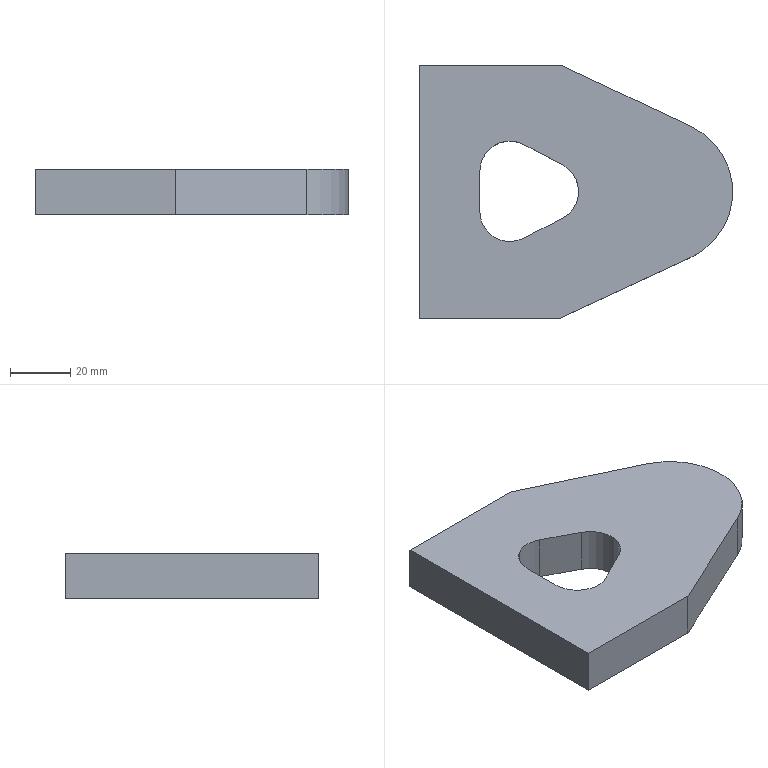Part | STEP file | ASND-0110-BAIF-08 | 1 solid | 16 faces | box 104 x 84 x 15 mm | volume 94605 mm3 | plane 10 | cylinder 6 | commonest cylinder face diameters 20 x5 48 x1
STEP:
#1=CARTESIAN_POINT('',(0.,0.,0.));
#2=DIRECTION('',(0.,0.,1.));
#3=DIRECTION('',(1.,0.,0.));
#4=AXIS2_PLACEMENT_3D('',#1,#2,#3);
#5=CARTESIAN_POINT('',(55.,6.858,20.));
#6=VERTEX_POINT('',#5);
#7=CARTESIAN_POINT('',(55.,6.858,5.));
#8=VERTEX_POINT('',#7);
#9=CARTESIAN_POINT('',(55.,6.858,0.));
#10=DIRECTION('',(0.,0.,-1.));
#11=VECTOR('',#10,1.);
#12=LINE('',#9,#11);
#13=CARTESIAN_POINT('',(65.,6.858,0.));
#14=DIRECTION('',(0.,0.,1.));
#15=DIRECTION('',(-0.5173,0.8558,0.));
#16=AXIS2_PLACEMENT_3D('',#13,#14,#15);
#17=CYLINDRICAL_SURFACE('',#16,10.);
#18=CARTESIAN_POINT('',(1.027,0.));
#19=DIRECTION('',(0.,-1.));
#20=VECTOR('',#19,1.);
#21=LINE('',#18,#20);
#22=(GEOMETRIC_REPRESENTATION_CONTEXT(2)PARAMETRIC_REPRESENTATION_CONTEXT()REPRESENTATION_CONTEXT('',''));
#23=DEFINITIONAL_REPRESENTATION('',(#21),#22);
#24=PCURVE('',#17,#23);
#25=CARTESIAN_POINT('',(55.,57.525,0.));
#26=DIRECTION('',(-1.,0.,0.));
#27=DIRECTION('',(0.,0.7071,0.7071));
#28=AXIS2_PLACEMENT_3D('',#25,#26,#27);
#29=PLANE('',#28);
#30=CARTESIAN_POINT('',(-35.827,-35.827));
#31=DIRECTION('',(-0.7071,0.7071));
#32=VECTOR('',#31,1.);
#33=LINE('',#30,#32);
#34=(GEOMETRIC_REPRESENTATION_CONTEXT(2)PARAMETRIC_REPRESENTATION_CONTEXT()REPRESENTATION_CONTEXT('',''));
#35=DEFINITIONAL_REPRESENTATION('',(#33),#34);
#36=PCURVE('',#29,#35);
#37=SURFACE_CURVE('',#12,(#24,#36),.PCURVE_S1.);
#38=EDGE_CURVE('',#6,#8,#37,.T.);
#39=ORIENTED_EDGE('',*,*,#38,.F.);
#40=CARTESIAN_POINT('',(59.827,15.416,20.));
#41=VERTEX_POINT('',#40);
#42=CARTESIAN_POINT('',(65.,6.858,20.));
#43=DIRECTION('',(0.,0.,1.));
#44=DIRECTION('',(-0.5173,0.8558,0.));
#45=AXIS2_PLACEMENT_3D('',#42,#43,#44);
#46=CIRCLE('',#45,10.);
#47=CARTESIAN_POINT('',(0.,20.));
#48=DIRECTION('',(1.,0.));
#49=VECTOR('',#48,1.);
#50=LINE('',#47,#49);
#51=(GEOMETRIC_REPRESENTATION_CONTEXT(2)PARAMETRIC_REPRESENTATION_CONTEXT()REPRESENTATION_CONTEXT('',''));
#52=DEFINITIONAL_REPRESENTATION('',(#50),#51);
#53=PCURVE('',#17,#52);
#54=CARTESIAN_POINT('',(115.,0.,20.));
#55=DIRECTION('',(0.,0.,1.));
#56=DIRECTION('',(0.7071,0.7071,0.));
#57=AXIS2_PLACEMENT_3D('',#54,#55,#56);
#58=PLANE('',#57);
#59=CARTESIAN_POINT('',(-30.506,40.205));
#60=DIRECTION('',(0.2394,0.9709));
#61=AXIS2_PLACEMENT_2D('',#59,#60);
#62=CIRCLE('',#61,10.);
#63=(GEOMETRIC_REPRESENTATION_CONTEXT(2)PARAMETRIC_REPRESENTATION_CONTEXT()REPRESENTATION_CONTEXT('',''));
#64=DEFINITIONAL_REPRESENTATION('',(#62),#63);
#65=PCURVE('',#58,#64);
#66=SURFACE_CURVE('',#46,(#53,#65),.PCURVE_S1.);
#67=EDGE_CURVE('',#41,#6,#66,.T.);
#68=ORIENTED_EDGE('',*,*,#67,.F.);
#69=CARTESIAN_POINT('',(59.827,15.416,5.));
#70=VERTEX_POINT('',#69);
#71=CARTESIAN_POINT('',(59.827,15.416,0.));
#72=DIRECTION('',(0.,0.,1.));
#73=VECTOR('',#72,1.);
#74=LINE('',#71,#73);
#75=CARTESIAN_POINT('',(0.,0.));
#76=DIRECTION('',(0.,1.));
#77=VECTOR('',#76,1.);
#78=LINE('',#75,#77);
#79=(GEOMETRIC_REPRESENTATION_CONTEXT(2)PARAMETRIC_REPRESENTATION_CONTEXT()REPRESENTATION_CONTEXT('',''));
#80=DEFINITIONAL_REPRESENTATION('',(#78),#79);
#81=PCURVE('',#17,#80);
#82=CARTESIAN_POINT('',(65.,6.858,0.));
#83=DIRECTION('',(0.,0.,1.));
#84=DIRECTION('',(-0.5173,0.8558,0.));
#85=AXIS2_PLACEMENT_3D('',#82,#83,#84);
#86=CYLINDRICAL_SURFACE('',#85,10.);
#87=CARTESIAN_POINT('',(6.283,0.));
#88=DIRECTION('',(0.,1.));
#89=VECTOR('',#88,1.);
#90=LINE('',#87,#89);
#91=(GEOMETRIC_REPRESENTATION_CONTEXT(2)PARAMETRIC_REPRESENTATION_CONTEXT()REPRESENTATION_CONTEXT('',''));
#92=DEFINITIONAL_REPRESENTATION('',(#90),#91);
#93=PCURVE('',#86,#92);
#94=SURFACE_CURVE('',#74,(#81,#93),.PCURVE_S1.);
#95=EDGE_CURVE('',#70,#41,#94,.T.);
#96=ORIENTED_EDGE('',*,*,#95,.F.);
#97=CARTESIAN_POINT('',(65.,6.858,5.));
#98=DIRECTION('',(0.,0.,-1.));
#99=DIRECTION('',(-0.5173,0.8558,0.));
#100=AXIS2_PLACEMENT_3D('',#97,#98,#99);
#101=CIRCLE('',#100,10.);
#102=CARTESIAN_POINT('',(6.283,5.));
#103=DIRECTION('',(-1.,0.));
#104=VECTOR('',#103,1.);
#105=LINE('',#102,#104);
#106=(GEOMETRIC_REPRESENTATION_CONTEXT(2)PARAMETRIC_REPRESENTATION_CONTEXT()REPRESENTATION_CONTEXT('',''));
#107=DEFINITIONAL_REPRESENTATION('',(#105),#106);
#108=PCURVE('',#17,#107);
#109=CARTESIAN_POINT('',(115.,0.,5.));
#110=DIRECTION('',(0.,0.,1.));
#111=DIRECTION('',(0.7071,0.7071,0.));
#112=AXIS2_PLACEMENT_3D('',#109,#110,#111);
#113=PLANE('',#112);
#114=CARTESIAN_POINT('',(-28.113,49.914));
#115=CARTESIAN_POINT('',(-11.296,45.768));
#116=CARTESIAN_POINT('',(-23.294,33.277));
#117=CARTESIAN_POINT('',(-35.293,20.786));
#118=CARTESIAN_POINT('',(-40.111,37.423));
#119=CARTESIAN_POINT('',(-44.93,54.06));
#120=CARTESIAN_POINT('',(-28.113,49.914));
#121=(BOUNDED_CURVE()B_SPLINE_CURVE(2,(#114,#115,#116,#117,#118,#119,#120),.UNSPECIFIED.,.T.,.F.)B_SPLINE_CURVE_WITH_KNOTS((1,2,2,2,2,1),(-2.094,0.,2.094,4.189,6.283,8.378),.UNSPECIFIED.)CURVE()GEOMETRIC_REPRESENTATION_ITEM()RATIONAL_B_SPLINE_CURVE((1.,0.5,1.,0.5,1.,0.5,1.))REPRESENTATION_ITEM(''));
#122=(GEOMETRIC_REPRESENTATION_CONTEXT(2)PARAMETRIC_REPRESENTATION_CONTEXT()REPRESENTATION_CONTEXT('',''));
#123=DEFINITIONAL_REPRESENTATION('',(#121),#122);
#124=PCURVE('',#113,#123);
#125=SURFACE_CURVE('',#101,(#108,#124),.PCURVE_S1.);
#126=EDGE_CURVE('',#8,#70,#125,.T.);
#127=ORIENTED_EDGE('',*,*,#126,.F.);
#128=EDGE_LOOP('',(#39,#68,#96,#127));
#129=FACE_BOUND('',#128,.F.);
#130=ADVANCED_FACE('',(#129),#17,.F.);
#131=CARTESIAN_POINT('',(55.,-6.459,5.));
#132=VERTEX_POINT('',#131);
#133=CARTESIAN_POINT('',(55.,-6.459,20.));
#134=VERTEX_POINT('',#133);
#135=CARTESIAN_POINT('',(55.,-6.459,0.));
#136=DIRECTION('',(0.,0.,1.));
#137=VECTOR('',#136,1.);
#138=LINE('',#135,#137);
#139=CARTESIAN_POINT('',(65.,-6.459,0.));
#140=DIRECTION('',(0.,0.,-1.));
#141=DIRECTION('',(-0.5205,-0.8539,0.));
#142=AXIS2_PLACEMENT_3D('',#139,#140,#141);
#143=CYLINDRICAL_SURFACE('',#142,10.);
#144=CARTESIAN_POINT('',(1.023,0.));
#145=DIRECTION('',(0.,-1.));
#146=VECTOR('',#145,1.);
#147=LINE('',#144,#146);
#148=(GEOMETRIC_REPRESENTATION_CONTEXT(2)PARAMETRIC_REPRESENTATION_CONTEXT()REPRESENTATION_CONTEXT('',''));
#149=DEFINITIONAL_REPRESENTATION('',(#147),#148);
#150=PCURVE('',#143,#149);
#151=CARTESIAN_POINT('',(-45.244,-45.244));
#152=DIRECTION('',(0.7071,-0.7071));
#153=VECTOR('',#152,1.);
#154=LINE('',#151,#153);
#155=(GEOMETRIC_REPRESENTATION_CONTEXT(2)PARAMETRIC_REPRESENTATION_CONTEXT()REPRESENTATION_CONTEXT('',''));
#156=DEFINITIONAL_REPRESENTATION('',(#154),#155);
#157=PCURVE('',#29,#156);
#158=SURFACE_CURVE('',#138,(#150,#157),.PCURVE_S1.);
#159=EDGE_CURVE('',#132,#134,#158,.T.);
#160=ORIENTED_EDGE('',*,*,#159,.F.);
#161=CARTESIAN_POINT('',(59.795,-14.998,5.));
#162=VERTEX_POINT('',#161);
#163=CARTESIAN_POINT('',(65.,-6.459,5.));
#164=DIRECTION('',(0.,0.,-1.));
#165=DIRECTION('',(-0.5205,-0.8539,0.));
#166=AXIS2_PLACEMENT_3D('',#163,#164,#165);
#167=CIRCLE('',#166,10.);
#168=CARTESIAN_POINT('',(0.,-5.));
#169=DIRECTION('',(1.,0.));
#170=VECTOR('',#169,1.);
#171=LINE('',#168,#170);
#172=(GEOMETRIC_REPRESENTATION_CONTEXT(2)PARAMETRIC_REPRESENTATION_CONTEXT()REPRESENTATION_CONTEXT('',''));
#173=DEFINITIONAL_REPRESENTATION('',(#171),#172);
#174=PCURVE('',#143,#173);
#175=CARTESIAN_POINT('',(-49.641,28.431));
#176=CARTESIAN_POINT('',(-53.724,45.263));
#177=CARTESIAN_POINT('',(-37.105,40.383));
#178=CARTESIAN_POINT('',(-20.486,35.502));
#179=CARTESIAN_POINT('',(-33.022,23.55));
#180=CARTESIAN_POINT('',(-45.558,11.598));
#181=CARTESIAN_POINT('',(-49.641,28.431));
#182=(BOUNDED_CURVE()B_SPLINE_CURVE(2,(#175,#176,#177,#178,#179,#180,#181),.UNSPECIFIED.,.T.,.F.)B_SPLINE_CURVE_WITH_KNOTS((1,2,2,2,2,1),(-2.094,0.,2.094,4.189,6.283,8.378),.UNSPECIFIED.)CURVE()GEOMETRIC_REPRESENTATION_ITEM()RATIONAL_B_SPLINE_CURVE((1.,0.5,1.,0.5,1.,0.5,1.))REPRESENTATION_ITEM(''));
#183=(GEOMETRIC_REPRESENTATION_CONTEXT(2)PARAMETRIC_REPRESENTATION_CONTEXT()REPRESENTATION_CONTEXT('',''));
#184=DEFINITIONAL_REPRESENTATION('',(#182),#183);
#185=PCURVE('',#113,#184);
#186=SURFACE_CURVE('',#167,(#174,#185),.PCURVE_S1.);
#187=EDGE_CURVE('',#162,#132,#186,.T.);
#188=ORIENTED_EDGE('',*,*,#187,.F.);
#189=CARTESIAN_POINT('',(59.795,-14.998,20.));
#190=VERTEX_POINT('',#189);
#191=CARTESIAN_POINT('',(59.795,-14.998,0.));
#192=DIRECTION('',(0.,0.,-1.));
#193=VECTOR('',#192,1.);
#194=LINE('',#191,#193);
#195=CARTESIAN_POINT('',(0.,0.));
#196=DIRECTION('',(0.,1.));
#197=VECTOR('',#196,1.);
#198=LINE('',#195,#197);
#199=(GEOMETRIC_REPRESENTATION_CONTEXT(2)PARAMETRIC_REPRESENTATION_CONTEXT()REPRESENTATION_CONTEXT('',''));
#200=DEFINITIONAL_REPRESENTATION('',(#198),#199);
#201=PCURVE('',#143,#200);
#202=CARTESIAN_POINT('',(65.,-6.459,0.));
#203=DIRECTION('',(0.,0.,-1.));
#204=DIRECTION('',(-0.5205,-0.8539,0.));
#205=AXIS2_PLACEMENT_3D('',#202,#203,#204);
#206=CYLINDRICAL_SURFACE('',#205,10.);
#207=CARTESIAN_POINT('',(6.283,0.));
#208=DIRECTION('',(0.,1.));
#209=VECTOR('',#208,1.);
#210=LINE('',#207,#209);
#211=(GEOMETRIC_REPRESENTATION_CONTEXT(2)PARAMETRIC_REPRESENTATION_CONTEXT()REPRESENTATION_CONTEXT('',''));
#212=DEFINITIONAL_REPRESENTATION('',(#210),#211);
#213=PCURVE('',#206,#212);
#214=SURFACE_CURVE('',#194,(#201,#213),.PCURVE_S1.);
#215=EDGE_CURVE('',#190,#162,#214,.T.);
#216=ORIENTED_EDGE('',*,*,#215,.F.);
#217=CARTESIAN_POINT('',(65.,-6.459,20.));
#218=DIRECTION('',(0.,0.,1.));
#219=DIRECTION('',(-0.5205,-0.8539,0.));
#220=AXIS2_PLACEMENT_3D('',#217,#218,#219);
#221=CIRCLE('',#220,10.);
#222=CARTESIAN_POINT('',(6.283,-20.));
#223=DIRECTION('',(-1.,0.));
#224=VECTOR('',#223,1.);
#225=LINE('',#222,#224);
#226=(GEOMETRIC_REPRESENTATION_CONTEXT(2)PARAMETRIC_REPRESENTATION_CONTEXT()REPRESENTATION_CONTEXT('',''));
#227=DEFINITIONAL_REPRESENTATION('',(#225),#226);
#228=PCURVE('',#143,#227);
#229=CARTESIAN_POINT('',(-39.923,30.788));
#230=DIRECTION('',(-0.9718,-0.2357));
#231=AXIS2_PLACEMENT_2D('',#229,#230);
#232=CIRCLE('',#231,10.);
#233=(GEOMETRIC_REPRESENTATION_CONTEXT(2)PARAMETRIC_REPRESENTATION_CONTEXT()REPRESENTATION_CONTEXT('',''));
#234=DEFINITIONAL_REPRESENTATION('',(#232),#233);
#235=PCURVE('',#58,#234);
#236=SURFACE_CURVE('',#221,(#228,#235),.PCURVE_S1.);
#237=EDGE_CURVE('',#134,#190,#236,.T.);
#238=ORIENTED_EDGE('',*,*,#237,.F.);
#239=EDGE_LOOP('',(#160,#188,#216,#238));
#240=FACE_BOUND('',#239,.F.);
#241=ADVANCED_FACE('',(#240),#143,.F.);
#242=CARTESIAN_POINT('',(82.175,42.,20.));
#243=VERTEX_POINT('',#242);
#244=CARTESIAN_POINT('',(125.231,21.71,20.));
#245=VERTEX_POINT('',#244);
#246=CARTESIAN_POINT('',(71.564,47.,20.));
#247=DIRECTION('',(0.9046,-0.4263,0.));
#248=VECTOR('',#247,1.);
#249=LINE('',#246,#248);
#250=CARTESIAN_POINT('',(71.564,47.,5.));
#251=DIRECTION('',(0.4263,0.9046,0.));
#252=DIRECTION('',(0.6708,-0.3161,0.6708));
#253=AXIS2_PLACEMENT_3D('',#250,#251,#252);
#254=PLANE('',#253);
#255=CARTESIAN_POINT('',(10.063,-11.124));
#256=DIRECTION('',(0.7416,0.6708));
#257=VECTOR('',#256,1.);
#258=LINE('',#255,#257);
#259=(GEOMETRIC_REPRESENTATION_CONTEXT(2)PARAMETRIC_REPRESENTATION_CONTEXT()REPRESENTATION_CONTEXT('',''));
#260=DEFINITIONAL_REPRESENTATION('',(#258),#259);
#261=PCURVE('',#254,#260);
#262=CARTESIAN_POINT('',(2.52,63.948));
#263=DIRECTION('',(0.3382,-0.9411));
#264=VECTOR('',#263,1.);
#265=LINE('',#262,#264);
#266=(GEOMETRIC_REPRESENTATION_CONTEXT(2)PARAMETRIC_REPRESENTATION_CONTEXT()REPRESENTATION_CONTEXT('',''));
#267=DEFINITIONAL_REPRESENTATION('',(#265),#266);
#268=PCURVE('',#58,#267);
#269=SURFACE_CURVE('',#249,(#261,#268),.PCURVE_S1.);
#270=EDGE_CURVE('',#243,#245,#269,.T.);
#271=ORIENTED_EDGE('',*,*,#270,.T.);
#272=CARTESIAN_POINT('',(125.231,21.71,5.));
#273=VERTEX_POINT('',#272);
#274=CARTESIAN_POINT('',(125.231,21.71,5.));
#275=DIRECTION('',(0.,0.,1.));
#276=VECTOR('',#275,1.);
#277=LINE('',#274,#276);
#278=CARTESIAN_POINT('',(43.997,39.799));
#279=DIRECTION('',(0.6708,-0.7416));
#280=VECTOR('',#279,1.);
#281=LINE('',#278,#280);
#282=(GEOMETRIC_REPRESENTATION_CONTEXT(2)PARAMETRIC_REPRESENTATION_CONTEXT()REPRESENTATION_CONTEXT('',''));
#283=DEFINITIONAL_REPRESENTATION('',(#281),#282);
#284=PCURVE('',#254,#283);
#285=CARTESIAN_POINT('',(115.,0.,5.));
#286=DIRECTION('',(0.,0.,1.));
#287=DIRECTION('',(-1.,0.,0.));
#288=AXIS2_PLACEMENT_3D('',#285,#286,#287);
#289=CYLINDRICAL_SURFACE('',#288,24.);
#290=CARTESIAN_POINT('',(4.272,0.));
#291=DIRECTION('',(0.,1.));
#292=VECTOR('',#291,1.);
#293=LINE('',#290,#292);
#294=(GEOMETRIC_REPRESENTATION_CONTEXT(2)PARAMETRIC_REPRESENTATION_CONTEXT()REPRESENTATION_CONTEXT('',''));
#295=DEFINITIONAL_REPRESENTATION('',(#293),#294);
#296=PCURVE('',#289,#295);
#297=SURFACE_CURVE('',#277,(#284,#296),.PCURVE_S1.);
#298=EDGE_CURVE('',#273,#245,#297,.T.);
#299=ORIENTED_EDGE('',*,*,#298,.F.);
#300=CARTESIAN_POINT('',(82.175,42.,5.));
#301=VERTEX_POINT('',#300);
#302=CARTESIAN_POINT('',(71.564,47.,5.));
#303=DIRECTION('',(0.9046,-0.4263,0.));
#304=VECTOR('',#303,1.);
#305=LINE('',#302,#304);
#306=CARTESIAN_POINT('',(0.,0.));
#307=DIRECTION('',(0.7416,0.6708));
#308=VECTOR('',#307,1.);
#309=LINE('',#306,#308);
#310=(GEOMETRIC_REPRESENTATION_CONTEXT(2)PARAMETRIC_REPRESENTATION_CONTEXT()REPRESENTATION_CONTEXT('',''));
#311=DEFINITIONAL_REPRESENTATION('',(#309),#310);
#312=PCURVE('',#254,#311);
#313=CARTESIAN_POINT('',(2.52,63.948));
#314=DIRECTION('',(0.3382,-0.9411));
#315=VECTOR('',#314,1.);
#316=LINE('',#313,#315);
#317=(GEOMETRIC_REPRESENTATION_CONTEXT(2)PARAMETRIC_REPRESENTATION_CONTEXT()REPRESENTATION_CONTEXT('',''));
#318=DEFINITIONAL_REPRESENTATION('',(#316),#317);
#319=PCURVE('',#113,#318);
#320=SURFACE_CURVE('',#305,(#312,#319),.PCURVE_S1.);
#321=EDGE_CURVE('',#301,#273,#320,.T.);
#322=ORIENTED_EDGE('',*,*,#321,.F.);
#323=CARTESIAN_POINT('',(82.175,42.,12.5));
#324=DIRECTION('',(0.,0.,-1.));
#325=VECTOR('',#324,1.);
#326=LINE('',#323,#325);
#327=CARTESIAN_POINT('',(13.73,2.307));
#328=DIRECTION('',(-0.6708,0.7416));
#329=VECTOR('',#328,1.);
#330=LINE('',#327,#329);
#331=(GEOMETRIC_REPRESENTATION_CONTEXT(2)PARAMETRIC_REPRESENTATION_CONTEXT()REPRESENTATION_CONTEXT('',''));
#332=DEFINITIONAL_REPRESENTATION('',(#330),#331);
#333=PCURVE('',#254,#332);
#334=CARTESIAN_POINT('',(10.,42.,20.));
#335=DIRECTION('',(0.,-1.,0.));
#336=DIRECTION('',(0.7071,0.,0.7071));
#337=AXIS2_PLACEMENT_3D('',#334,#335,#336);
#338=PLANE('',#337);
#339=CARTESIAN_POINT('',(45.732,-56.339));
#340=DIRECTION('',(-0.7071,-0.7071));
#341=VECTOR('',#340,1.);
#342=LINE('',#339,#341);
#343=(GEOMETRIC_REPRESENTATION_CONTEXT(2)PARAMETRIC_REPRESENTATION_CONTEXT()REPRESENTATION_CONTEXT('',''));
#344=DEFINITIONAL_REPRESENTATION('',(#342),#343);
#345=PCURVE('',#338,#344);
#346=SURFACE_CURVE('',#326,(#333,#345),.PCURVE_S1.);
#347=EDGE_CURVE('',#243,#301,#346,.T.);
#348=ORIENTED_EDGE('',*,*,#347,.F.);
#349=EDGE_LOOP('',(#271,#299,#322,#348));
#350=FACE_BOUND('',#349,.T.);
#351=ADVANCED_FACE('',(#350),#254,.T.);
#352=CARTESIAN_POINT('',(125.104,-21.77,20.));
#353=VERTEX_POINT('',#352);
#354=CARTESIAN_POINT('',(115.,0.,20.));
#355=DIRECTION('',(0.,0.,-1.));
#356=DIRECTION('',(-1.,0.,0.));
#357=AXIS2_PLACEMENT_3D('',#354,#355,#356);
#358=CIRCLE('',#357,24.);
#359=CARTESIAN_POINT('',(6.283,15.));
#360=DIRECTION('',(-1.,0.));
#361=VECTOR('',#360,1.);
#362=LINE('',#359,#361);
#363=(GEOMETRIC_REPRESENTATION_CONTEXT(2)PARAMETRIC_REPRESENTATION_CONTEXT()REPRESENTATION_CONTEXT('',''));
#364=DEFINITIONAL_REPRESENTATION('',(#362),#363);
#365=PCURVE('',#289,#364);
#366=CARTESIAN_POINT('',(-16.971,16.971));
#367=CARTESIAN_POINT('',(12.423,46.364));
#368=CARTESIAN_POINT('',(23.182,6.212));
#369=CARTESIAN_POINT('',(33.941,-33.941));
#370=CARTESIAN_POINT('',(-6.212,-23.182));
#371=CARTESIAN_POINT('',(-46.364,-12.423));
#372=CARTESIAN_POINT('',(-16.971,16.971));
#373=(BOUNDED_CURVE()B_SPLINE_CURVE(2,(#366,#367,#368,#369,#370,#371,#372),.UNSPECIFIED.,.T.,.F.)B_SPLINE_CURVE_WITH_KNOTS((1,2,2,2,2,1),(-2.094,0.,2.094,4.189,6.283,8.378),.UNSPECIFIED.)CURVE()GEOMETRIC_REPRESENTATION_ITEM()RATIONAL_B_SPLINE_CURVE((1.,0.5,1.,0.5,1.,0.5,1.))REPRESENTATION_ITEM(''));
#374=(GEOMETRIC_REPRESENTATION_CONTEXT(2)PARAMETRIC_REPRESENTATION_CONTEXT()REPRESENTATION_CONTEXT('',''));
#375=DEFINITIONAL_REPRESENTATION('',(#373),#374);
#376=PCURVE('',#58,#375);
#377=SURFACE_CURVE('',#358,(#365,#376),.PCURVE_S1.);
#378=EDGE_CURVE('',#245,#353,#377,.T.);
#379=ORIENTED_EDGE('',*,*,#378,.T.);
#380=CARTESIAN_POINT('',(125.104,-21.77,5.));
#381=VERTEX_POINT('',#380);
#382=CARTESIAN_POINT('',(125.104,-21.77,5.));
#383=DIRECTION('',(0.,0.,1.));
#384=VECTOR('',#383,1.);
#385=LINE('',#382,#384);
#386=CARTESIAN_POINT('',(2.005,0.));
#387=DIRECTION('',(0.,1.));
#388=VECTOR('',#387,1.);
#389=LINE('',#386,#388);
#390=(GEOMETRIC_REPRESENTATION_CONTEXT(2)PARAMETRIC_REPRESENTATION_CONTEXT()REPRESENTATION_CONTEXT('',''));
#391=DEFINITIONAL_REPRESENTATION('',(#389),#390);
#392=PCURVE('',#289,#391);
#393=CARTESIAN_POINT('',(125.104,-21.77,5.));
#394=DIRECTION('',(0.421,-0.9071,0.));
#395=DIRECTION('',(0.6719,0.3118,0.6719));
#396=AXIS2_PLACEMENT_3D('',#393,#394,#395);
#397=PLANE('',#396);
#398=CARTESIAN_POINT('',(0.,0.));
#399=DIRECTION('',(0.6719,0.7407));
#400=VECTOR('',#399,1.);
#401=LINE('',#398,#400);
#402=(GEOMETRIC_REPRESENTATION_CONTEXT(2)PARAMETRIC_REPRESENTATION_CONTEXT()REPRESENTATION_CONTEXT('',''));
#403=DEFINITIONAL_REPRESENTATION('',(#401),#402);
#404=PCURVE('',#397,#403);
#405=SURFACE_CURVE('',#385,(#392,#404),.PCURVE_S1.);
#406=EDGE_CURVE('',#381,#353,#405,.T.);
#407=ORIENTED_EDGE('',*,*,#406,.F.);
#408=CARTESIAN_POINT('',(115.,0.,5.));
#409=DIRECTION('',(0.,0.,-1.));
#410=DIRECTION('',(-1.,0.,0.));
#411=AXIS2_PLACEMENT_3D('',#408,#409,#410);
#412=CIRCLE('',#411,24.);
#413=CARTESIAN_POINT('',(6.283,0.));
#414=DIRECTION('',(-1.,0.));
#415=VECTOR('',#414,1.);
#416=LINE('',#413,#415);
#417=(GEOMETRIC_REPRESENTATION_CONTEXT(2)PARAMETRIC_REPRESENTATION_CONTEXT()REPRESENTATION_CONTEXT('',''));
#418=DEFINITIONAL_REPRESENTATION('',(#416),#417);
#419=PCURVE('',#289,#418);
#420=CARTESIAN_POINT('',(-16.971,16.971));
#421=CARTESIAN_POINT('',(12.423,46.364));
#422=CARTESIAN_POINT('',(23.182,6.212));
#423=CARTESIAN_POINT('',(33.941,-33.941));
#424=CARTESIAN_POINT('',(-6.212,-23.182));
#425=CARTESIAN_POINT('',(-46.364,-12.423));
#426=CARTESIAN_POINT('',(-16.971,16.971));
#427=(BOUNDED_CURVE()B_SPLINE_CURVE(2,(#420,#421,#422,#423,#424,#425,#426),.UNSPECIFIED.,.T.,.F.)B_SPLINE_CURVE_WITH_KNOTS((1,2,2,2,2,1),(-2.094,0.,2.094,4.189,6.283,8.378),.UNSPECIFIED.)CURVE()GEOMETRIC_REPRESENTATION_ITEM()RATIONAL_B_SPLINE_CURVE((1.,0.5,1.,0.5,1.,0.5,1.))REPRESENTATION_ITEM(''));
#428=(GEOMETRIC_REPRESENTATION_CONTEXT(2)PARAMETRIC_REPRESENTATION_CONTEXT()REPRESENTATION_CONTEXT('',''));
#429=DEFINITIONAL_REPRESENTATION('',(#427),#428);
#430=PCURVE('',#113,#429);
#431=SURFACE_CURVE('',#412,(#419,#430),.PCURVE_S1.);
#432=EDGE_CURVE('',#273,#381,#431,.T.);
#433=ORIENTED_EDGE('',*,*,#432,.F.);
#434=ORIENTED_EDGE('',*,*,#298,.T.);
#435=EDGE_LOOP('',(#379,#407,#433,#434));
#436=FACE_BOUND('',#435,.T.);
#437=ADVANCED_FACE('',(#436),#289,.T.);
#438=CARTESIAN_POINT('',(81.515,-42.,20.));
#439=VERTEX_POINT('',#438);
#440=CARTESIAN_POINT('',(125.104,-21.77,20.));
#441=DIRECTION('',(-0.9071,-0.421,0.));
#442=VECTOR('',#441,1.);
#443=LINE('',#440,#442);
#444=CARTESIAN_POINT('',(10.078,11.11));
#445=DIRECTION('',(-0.7407,0.6719));
#446=VECTOR('',#445,1.);
#447=LINE('',#444,#446);
#448=(GEOMETRIC_REPRESENTATION_CONTEXT(2)PARAMETRIC_REPRESENTATION_CONTEXT()REPRESENTATION_CONTEXT('',''));
#449=DEFINITIONAL_REPRESENTATION('',(#447),#448);
#450=PCURVE('',#397,#449);
#451=CARTESIAN_POINT('',(-8.249,-22.538));
#452=DIRECTION('',(-0.9391,0.3437));
#453=VECTOR('',#452,1.);
#454=LINE('',#451,#453);
#455=(GEOMETRIC_REPRESENTATION_CONTEXT(2)PARAMETRIC_REPRESENTATION_CONTEXT()REPRESENTATION_CONTEXT('',''));
#456=DEFINITIONAL_REPRESENTATION('',(#454),#455);
#457=PCURVE('',#58,#456);
#458=SURFACE_CURVE('',#443,(#450,#457),.PCURVE_S1.);
#459=EDGE_CURVE('',#353,#439,#458,.T.);
#460=ORIENTED_EDGE('',*,*,#459,.T.);
#461=CARTESIAN_POINT('',(81.515,-42.,5.));
#462=VERTEX_POINT('',#461);
#463=CARTESIAN_POINT('',(81.515,-42.,12.5));
#464=DIRECTION('',(0.,0.,1.));
#465=VECTOR('',#464,1.);
#466=LINE('',#463,#465);
#467=CARTESIAN_POINT('',(-30.554,37.841));
#468=DIRECTION('',(0.6719,0.7407));
#469=VECTOR('',#468,1.);
#470=LINE('',#467,#469);
#471=(GEOMETRIC_REPRESENTATION_CONTEXT(2)PARAMETRIC_REPRESENTATION_CONTEXT()REPRESENTATION_CONTEXT('',''));
#472=DEFINITIONAL_REPRESENTATION('',(#470),#471);
#473=PCURVE('',#397,#472);
#474=CARTESIAN_POINT('',(10.,-42.,20.));
#475=DIRECTION('',(0.,1.,0.));
#476=DIRECTION('',(0.7071,0.,0.7071));
#477=AXIS2_PLACEMENT_3D('',#474,#475,#476);
#478=PLANE('',#477);
#479=CARTESIAN_POINT('',(45.266,55.872));
#480=DIRECTION('',(0.7071,-0.7071));
#481=VECTOR('',#480,1.);
#482=LINE('',#479,#481);
#483=(GEOMETRIC_REPRESENTATION_CONTEXT(2)PARAMETRIC_REPRESENTATION_CONTEXT()REPRESENTATION_CONTEXT('',''));
#484=DEFINITIONAL_REPRESENTATION('',(#482),#483);
#485=PCURVE('',#478,#484);
#486=SURFACE_CURVE('',#466,(#473,#485),.PCURVE_S1.);
#487=EDGE_CURVE('',#462,#439,#486,.T.);
#488=ORIENTED_EDGE('',*,*,#487,.F.);
#489=CARTESIAN_POINT('',(125.104,-21.77,5.));
#490=DIRECTION('',(-0.9071,-0.421,0.));
#491=VECTOR('',#490,1.);
#492=LINE('',#489,#491);
#493=CARTESIAN_POINT('',(0.,0.));
#494=DIRECTION('',(-0.7407,0.6719));
#495=VECTOR('',#494,1.);
#496=LINE('',#493,#495);
#497=(GEOMETRIC_REPRESENTATION_CONTEXT(2)PARAMETRIC_REPRESENTATION_CONTEXT()REPRESENTATION_CONTEXT('',''));
#498=DEFINITIONAL_REPRESENTATION('',(#496),#497);
#499=PCURVE('',#397,#498);
#500=CARTESIAN_POINT('',(-8.249,-22.538));
#501=DIRECTION('',(-0.9391,0.3437));
#502=VECTOR('',#501,1.);
#503=LINE('',#500,#502);
#504=(GEOMETRIC_REPRESENTATION_CONTEXT(2)PARAMETRIC_REPRESENTATION_CONTEXT()REPRESENTATION_CONTEXT('',''));
#505=DEFINITIONAL_REPRESENTATION('',(#503),#504);
#506=PCURVE('',#113,#505);
#507=SURFACE_CURVE('',#492,(#499,#506),.PCURVE_S1.);
#508=EDGE_CURVE('',#381,#462,#507,.T.);
#509=ORIENTED_EDGE('',*,*,#508,.F.);
#510=ORIENTED_EDGE('',*,*,#406,.T.);
#511=EDGE_LOOP('',(#460,#488,#509,#510));
#512=FACE_BOUND('',#511,.T.);
#513=ADVANCED_FACE('',(#512),#397,.T.);
#514=CARTESIAN_POINT('',(35.,-42.,5.));
#515=VERTEX_POINT('',#514);
#516=CARTESIAN_POINT('',(15.,-42.,5.));
#517=DIRECTION('',(1.,0.,0.));
#518=VECTOR('',#517,1.);
#519=LINE('',#516,#518);
#520=CARTESIAN_POINT('',(-7.071,14.142));
#521=DIRECTION('',(0.7071,0.7071));
#522=VECTOR('',#521,1.);
#523=LINE('',#520,#522);
#524=(GEOMETRIC_REPRESENTATION_CONTEXT(2)PARAMETRIC_REPRESENTATION_CONTEXT()REPRESENTATION_CONTEXT('',''));
#525=DEFINITIONAL_REPRESENTATION('',(#523),#524);
#526=PCURVE('',#478,#525);
#527=CARTESIAN_POINT('',(-100.409,41.012));
#528=DIRECTION('',(0.7071,-0.7071));
#529=VECTOR('',#528,1.);
#530=LINE('',#527,#529);
#531=(GEOMETRIC_REPRESENTATION_CONTEXT(2)PARAMETRIC_REPRESENTATION_CONTEXT()REPRESENTATION_CONTEXT('',''));
#532=DEFINITIONAL_REPRESENTATION('',(#530),#531);
#533=PCURVE('',#113,#532);
#534=SURFACE_CURVE('',#519,(#526,#533),.PCURVE_S1.);
#535=EDGE_CURVE('',#515,#462,#534,.T.);
#536=ORIENTED_EDGE('',*,*,#535,.T.);
#537=ORIENTED_EDGE('',*,*,#487,.T.);
#538=CARTESIAN_POINT('',(35.,-42.,20.));
#539=VERTEX_POINT('',#538);
#540=CARTESIAN_POINT('',(15.,-42.,20.));
#541=DIRECTION('',(1.,0.,0.));
#542=VECTOR('',#541,1.);
#543=LINE('',#540,#542);
#544=CARTESIAN_POINT('',(3.536,3.536));
#545=DIRECTION('',(0.7071,0.7071));
#546=VECTOR('',#545,1.);
#547=LINE('',#544,#546);
#548=(GEOMETRIC_REPRESENTATION_CONTEXT(2)PARAMETRIC_REPRESENTATION_CONTEXT()REPRESENTATION_CONTEXT('',''));
#549=DEFINITIONAL_REPRESENTATION('',(#547),#548);
#550=PCURVE('',#478,#549);
#551=CARTESIAN_POINT('',(-100.409,41.012));
#552=DIRECTION('',(0.7071,-0.7071));
#553=VECTOR('',#552,1.);
#554=LINE('',#551,#553);
#555=(GEOMETRIC_REPRESENTATION_CONTEXT(2)PARAMETRIC_REPRESENTATION_CONTEXT()REPRESENTATION_CONTEXT('',''));
#556=DEFINITIONAL_REPRESENTATION('',(#554),#555);
#557=PCURVE('',#58,#556);
#558=SURFACE_CURVE('',#543,(#550,#557),.PCURVE_S1.);
#559=EDGE_CURVE('',#539,#439,#558,.T.);
#560=ORIENTED_EDGE('',*,*,#559,.F.);
#561=CARTESIAN_POINT('',(35.,-42.,20.));
#562=DIRECTION('',(0.,0.,-1.));
#563=VECTOR('',#562,1.);
#564=LINE('',#561,#563);
#565=CARTESIAN_POINT('',(17.678,17.678));
#566=DIRECTION('',(-0.7071,0.7071));
#567=VECTOR('',#566,1.);
#568=LINE('',#565,#567);
#569=(GEOMETRIC_REPRESENTATION_CONTEXT(2)PARAMETRIC_REPRESENTATION_CONTEXT()REPRESENTATION_CONTEXT('',''));
#570=DEFINITIONAL_REPRESENTATION('',(#568),#569);
#571=PCURVE('',#478,#570);
#572=CARTESIAN_POINT('',(35.,-68.,20.));
#573=DIRECTION('',(1.,0.,0.));
#574=DIRECTION('',(0.,0.7071,0.7071));
#575=AXIS2_PLACEMENT_3D('',#572,#573,#574);
#576=PLANE('',#575);
#577=CARTESIAN_POINT('',(18.385,-18.385));
#578=DIRECTION('',(-0.7071,-0.7071));
#579=VECTOR('',#578,1.);
#580=LINE('',#577,#579);
#581=(GEOMETRIC_REPRESENTATION_CONTEXT(2)PARAMETRIC_REPRESENTATION_CONTEXT()REPRESENTATION_CONTEXT('',''));
#582=DEFINITIONAL_REPRESENTATION('',(#580),#581);
#583=PCURVE('',#576,#582);
#584=SURFACE_CURVE('',#564,(#571,#583),.PCURVE_S1.);
#585=EDGE_CURVE('',#539,#515,#584,.T.);
#586=ORIENTED_EDGE('',*,*,#585,.T.);
#587=EDGE_LOOP('',(#536,#537,#560,#586));
#588=FACE_BOUND('',#587,.T.);
#589=ADVANCED_FACE('',(#588),#478,.F.);
#590=CARTESIAN_POINT('',(69.582,-15.348,5.));
#591=VERTEX_POINT('',#590);
#592=CARTESIAN_POINT('',(82.382,-8.75,5.));
#593=VERTEX_POINT('',#592);
#594=CARTESIAN_POINT('',(44.582,-28.234,5.));
#595=DIRECTION('',(0.8889,0.4582,0.));
#596=VECTOR('',#595,1.);
#597=LINE('',#594,#596);
#598=CARTESIAN_POINT('',(-69.758,29.829));
#599=DIRECTION('',(0.9525,-0.3046));
#600=VECTOR('',#599,1.);
#601=LINE('',#598,#600);
#602=(GEOMETRIC_REPRESENTATION_CONTEXT(2)PARAMETRIC_REPRESENTATION_CONTEXT()REPRESENTATION_CONTEXT('',''));
#603=DEFINITIONAL_REPRESENTATION('',(#601),#602);
#604=PCURVE('',#113,#603);
#605=CARTESIAN_POINT('',(30.,-35.75,0.));
#606=DIRECTION('',(0.4582,-0.8889,0.));
#607=DIRECTION('',(0.6644,0.3424,0.6644));
#608=AXIS2_PLACEMENT_3D('',#605,#606,#607);
#609=PLANE('',#608);
#610=CARTESIAN_POINT('',(15.583,-7.161));
#611=DIRECTION('',(0.7474,-0.6644));
#612=VECTOR('',#611,1.);
#613=LINE('',#610,#612);
#614=(GEOMETRIC_REPRESENTATION_CONTEXT(2)PARAMETRIC_REPRESENTATION_CONTEXT()REPRESENTATION_CONTEXT('',''));
#615=DEFINITIONAL_REPRESENTATION('',(#613),#614);
#616=PCURVE('',#609,#615);
#617=SURFACE_CURVE('',#597,(#604,#616),.PCURVE_S1.);
#618=EDGE_CURVE('',#591,#593,#617,.T.);
#619=ORIENTED_EDGE('',*,*,#618,.T.);
#620=CARTESIAN_POINT('',(82.448,8.993,5.));
#621=VERTEX_POINT('',#620);
#622=CARTESIAN_POINT('',(77.8,0.1384,5.));
#623=DIRECTION('',(0.,0.,1.));
#624=DIRECTION('',(0.4648,0.8854,0.));
#625=AXIS2_PLACEMENT_3D('',#622,#623,#624);
#626=CIRCLE('',#625,10.);
#627=CARTESIAN_POINT('',(-26.206,26.402));
#628=DIRECTION('',(0.9547,0.2974));
#629=AXIS2_PLACEMENT_2D('',#627,#628);
#630=CIRCLE('',#629,10.);
#631=(GEOMETRIC_REPRESENTATION_CONTEXT(2)PARAMETRIC_REPRESENTATION_CONTEXT()REPRESENTATION_CONTEXT('',''));
#632=DEFINITIONAL_REPRESENTATION('',(#630),#631);
#633=PCURVE('',#113,#632);
#634=CARTESIAN_POINT('',(77.8,0.1384,0.));
#635=DIRECTION('',(0.,0.,1.));
#636=DIRECTION('',(0.4648,0.8854,0.));
#637=AXIS2_PLACEMENT_3D('',#634,#635,#636);
#638=CYLINDRICAL_SURFACE('',#637,10.);
#639=CARTESIAN_POINT('',(0.,5.));
#640=DIRECTION('',(1.,0.));
#641=VECTOR('',#640,1.);
#642=LINE('',#639,#641);
#643=(GEOMETRIC_REPRESENTATION_CONTEXT(2)PARAMETRIC_REPRESENTATION_CONTEXT()REPRESENTATION_CONTEXT('',''));
#644=DEFINITIONAL_REPRESENTATION('',(#642),#643);
#645=PCURVE('',#638,#644);
#646=SURFACE_CURVE('',#626,(#633,#645),.PCURVE_S1.);
#647=EDGE_CURVE('',#593,#621,#646,.T.);
#648=ORIENTED_EDGE('',*,*,#647,.T.);
#649=CARTESIAN_POINT('',(69.648,15.712,5.));
#650=VERTEX_POINT('',#649);
#651=CARTESIAN_POINT('',(84.648,7.838,5.));
#652=DIRECTION('',(-0.8854,0.4648,0.));
#653=VECTOR('',#652,1.);
#654=LINE('',#651,#653);
#655=CARTESIAN_POINT('',(-15.92,27.004));
#656=DIRECTION('',(-0.2974,0.9547));
#657=VECTOR('',#656,1.);
#658=LINE('',#655,#657);
#659=(GEOMETRIC_REPRESENTATION_CONTEXT(2)PARAMETRIC_REPRESENTATION_CONTEXT()REPRESENTATION_CONTEXT('',''));
#660=DEFINITIONAL_REPRESENTATION('',(#658),#659);
#661=PCURVE('',#113,#660);
#662=CARTESIAN_POINT('',(90.,5.028,0.));
#663=DIRECTION('',(0.4648,0.8854,0.));
#664=DIRECTION('',(0.6629,-0.348,0.6629));
#665=AXIS2_PLACEMENT_3D('',#662,#663,#664);
#666=PLANE('',#665);
#667=CARTESIAN_POINT('',(-1.211,-7.751));
#668=DIRECTION('',(-0.7487,-0.6629));
#669=VECTOR('',#668,1.);
#670=LINE('',#667,#669);
#671=(GEOMETRIC_REPRESENTATION_CONTEXT(2)PARAMETRIC_REPRESENTATION_CONTEXT()REPRESENTATION_CONTEXT('',''));
#672=DEFINITIONAL_REPRESENTATION('',(#670),#671);
#673=PCURVE('',#666,#672);
#674=SURFACE_CURVE('',#654,(#661,#673),.PCURVE_S1.);
#675=EDGE_CURVE('',#621,#650,#674,.T.);
#676=ORIENTED_EDGE('',*,*,#675,.T.);
#677=CARTESIAN_POINT('',(65.,6.858,5.));
#678=DIRECTION('',(0.,0.,-1.));
#679=DIRECTION('',(-0.5173,0.8558,0.));
#680=AXIS2_PLACEMENT_3D('',#677,#678,#679);
#681=CIRCLE('',#680,10.);
#682=CARTESIAN_POINT('',(-28.113,49.914));
#683=CARTESIAN_POINT('',(-11.296,45.768));
#684=CARTESIAN_POINT('',(-23.294,33.277));
#685=CARTESIAN_POINT('',(-35.293,20.786));
#686=CARTESIAN_POINT('',(-40.111,37.423));
#687=CARTESIAN_POINT('',(-44.93,54.06));
#688=CARTESIAN_POINT('',(-28.113,49.914));
#689=(BOUNDED_CURVE()B_SPLINE_CURVE(2,(#682,#683,#684,#685,#686,#687,#688),.UNSPECIFIED.,.T.,.F.)B_SPLINE_CURVE_WITH_KNOTS((1,2,2,2,2,1),(-2.094,0.,2.094,4.189,6.283,8.378),.UNSPECIFIED.)CURVE()GEOMETRIC_REPRESENTATION_ITEM()RATIONAL_B_SPLINE_CURVE((1.,0.5,1.,0.5,1.,0.5,1.))REPRESENTATION_ITEM(''));
#690=(GEOMETRIC_REPRESENTATION_CONTEXT(2)PARAMETRIC_REPRESENTATION_CONTEXT()REPRESENTATION_CONTEXT('',''));
#691=DEFINITIONAL_REPRESENTATION('',(#689),#690);
#692=PCURVE('',#113,#691);
#693=CARTESIAN_POINT('',(6.283,5.));
#694=DIRECTION('',(-1.,0.));
#695=VECTOR('',#694,1.);
#696=LINE('',#693,#695);
#697=(GEOMETRIC_REPRESENTATION_CONTEXT(2)PARAMETRIC_REPRESENTATION_CONTEXT()REPRESENTATION_CONTEXT('',''));
#698=DEFINITIONAL_REPRESENTATION('',(#696),#697);
#699=PCURVE('',#86,#698);
#700=SURFACE_CURVE('',#681,(#692,#699),.PCURVE_S1.);
#701=EDGE_CURVE('',#70,#650,#700,.T.);
#702=ORIENTED_EDGE('',*,*,#701,.F.);
#703=ORIENTED_EDGE('',*,*,#126,.F.);
#704=CARTESIAN_POINT('',(55.,40.981,5.));
#705=DIRECTION('',(0.,-1.,0.));
#706=VECTOR('',#705,1.);
#707=LINE('',#704,#706);
#708=CARTESIAN_POINT('',(-13.448,71.405));
#709=DIRECTION('',(-0.7071,-0.7071));
#710=VECTOR('',#709,1.);
#711=LINE('',#708,#710);
#712=(GEOMETRIC_REPRESENTATION_CONTEXT(2)PARAMETRIC_REPRESENTATION_CONTEXT()REPRESENTATION_CONTEXT('',''));
#713=DEFINITIONAL_REPRESENTATION('',(#711),#712);
#714=PCURVE('',#113,#713);
#715=CARTESIAN_POINT('',(-8.162,-15.234));
#716=DIRECTION('',(-0.7071,-0.7071));
#717=VECTOR('',#716,1.);
#718=LINE('',#715,#717);
#719=(GEOMETRIC_REPRESENTATION_CONTEXT(2)PARAMETRIC_REPRESENTATION_CONTEXT()REPRESENTATION_CONTEXT('',''));
#720=DEFINITIONAL_REPRESENTATION('',(#718),#719);
#721=PCURVE('',#29,#720);
#722=SURFACE_CURVE('',#707,(#714,#721),.PCURVE_S1.);
#723=EDGE_CURVE('',#8,#132,#722,.T.);
#724=ORIENTED_EDGE('',*,*,#723,.T.);
#725=ORIENTED_EDGE('',*,*,#187,.F.);
#726=CARTESIAN_POINT('',(65.,-6.459,5.));
#727=DIRECTION('',(0.,0.,-1.));
#728=DIRECTION('',(-0.5205,-0.8539,0.));
#729=AXIS2_PLACEMENT_3D('',#726,#727,#728);
#730=CIRCLE('',#729,10.);
#731=CARTESIAN_POINT('',(-49.641,28.431));
#732=CARTESIAN_POINT('',(-53.724,45.263));
#733=CARTESIAN_POINT('',(-37.105,40.383));
#734=CARTESIAN_POINT('',(-20.486,35.502));
#735=CARTESIAN_POINT('',(-33.022,23.55));
#736=CARTESIAN_POINT('',(-45.558,11.598));
#737=CARTESIAN_POINT('',(-49.641,28.431));
#738=(BOUNDED_CURVE()B_SPLINE_CURVE(2,(#731,#732,#733,#734,#735,#736,#737),.UNSPECIFIED.,.T.,.F.)B_SPLINE_CURVE_WITH_KNOTS((1,2,2,2,2,1),(-2.094,0.,2.094,4.189,6.283,8.378),.UNSPECIFIED.)CURVE()GEOMETRIC_REPRESENTATION_ITEM()RATIONAL_B_SPLINE_CURVE((1.,0.5,1.,0.5,1.,0.5,1.))REPRESENTATION_ITEM(''));
#739=(GEOMETRIC_REPRESENTATION_CONTEXT(2)PARAMETRIC_REPRESENTATION_CONTEXT()REPRESENTATION_CONTEXT('',''));
#740=DEFINITIONAL_REPRESENTATION('',(#738),#739);
#741=PCURVE('',#113,#740);
#742=CARTESIAN_POINT('',(0.,-5.));
#743=DIRECTION('',(1.,0.));
#744=VECTOR('',#743,1.);
#745=LINE('',#742,#744);
#746=(GEOMETRIC_REPRESENTATION_CONTEXT(2)PARAMETRIC_REPRESENTATION_CONTEXT()REPRESENTATION_CONTEXT('',''));
#747=DEFINITIONAL_REPRESENTATION('',(#745),#746);
#748=PCURVE('',#206,#747);
#749=SURFACE_CURVE('',#730,(#741,#748),.PCURVE_S1.);
#750=EDGE_CURVE('',#591,#162,#749,.T.);
#751=ORIENTED_EDGE('',*,*,#750,.F.);
#752=EDGE_LOOP('',(#619,#648,#676,#702,#703,#724,#725,#751));
#753=FACE_BOUND('',#752,.T.);
#754=ORIENTED_EDGE('',*,*,#321,.T.);
#755=ORIENTED_EDGE('',*,*,#432,.T.);
#756=ORIENTED_EDGE('',*,*,#508,.T.);
#757=ORIENTED_EDGE('',*,*,#535,.F.);
#758=CARTESIAN_POINT('',(35.,42.,5.));
#759=VERTEX_POINT('',#758);
#760=CARTESIAN_POINT('',(35.,63.,5.));
#761=DIRECTION('',(0.,-1.,0.));
#762=VECTOR('',#761,1.);
#763=LINE('',#760,#762);
#764=CARTESIAN_POINT('',(-12.021,101.116));
#765=DIRECTION('',(-0.7071,-0.7071));
#766=VECTOR('',#765,1.);
#767=LINE('',#764,#766);
#768=(GEOMETRIC_REPRESENTATION_CONTEXT(2)PARAMETRIC_REPRESENTATION_CONTEXT()REPRESENTATION_CONTEXT('',''));
#769=DEFINITIONAL_REPRESENTATION('',(#767),#768);
#770=PCURVE('',#113,#769);
#771=CARTESIAN_POINT('',(82.024,-103.238));
#772=DIRECTION('',(-0.7071,0.7071));
#773=VECTOR('',#772,1.);
#774=LINE('',#771,#773);
#775=(GEOMETRIC_REPRESENTATION_CONTEXT(2)PARAMETRIC_REPRESENTATION_CONTEXT()REPRESENTATION_CONTEXT('',''));
#776=DEFINITIONAL_REPRESENTATION('',(#774),#775);
#777=PCURVE('',#576,#776);
#778=SURFACE_CURVE('',#763,(#770,#777),.PCURVE_S1.);
#779=EDGE_CURVE('',#759,#515,#778,.T.);
#780=ORIENTED_EDGE('',*,*,#779,.F.);
#781=CARTESIAN_POINT('',(53.49,42.,5.));
#782=DIRECTION('',(-1.,0.,0.));
#783=VECTOR('',#782,1.);
#784=LINE('',#781,#783);
#785=CARTESIAN_POINT('',(-13.796,73.193));
#786=DIRECTION('',(-0.7071,0.7071));
#787=VECTOR('',#786,1.);
#788=LINE('',#785,#787);
#789=(GEOMETRIC_REPRESENTATION_CONTEXT(2)PARAMETRIC_REPRESENTATION_CONTEXT()REPRESENTATION_CONTEXT('',''));
#790=DEFINITIONAL_REPRESENTATION('',(#788),#789);
#791=PCURVE('',#113,#790);
#792=CARTESIAN_POINT('',(20.145,-41.358));
#793=DIRECTION('',(-0.7071,0.7071));
#794=VECTOR('',#793,1.);
#795=LINE('',#792,#794);
#796=(GEOMETRIC_REPRESENTATION_CONTEXT(2)PARAMETRIC_REPRESENTATION_CONTEXT()REPRESENTATION_CONTEXT('',''));
#797=DEFINITIONAL_REPRESENTATION('',(#795),#796);
#798=PCURVE('',#338,#797);
#799=SURFACE_CURVE('',#784,(#791,#798),.PCURVE_S1.);
#800=EDGE_CURVE('',#301,#759,#799,.T.);
#801=ORIENTED_EDGE('',*,*,#800,.F.);
#802=EDGE_LOOP('',(#754,#755,#756,#757,#780,#801));
#803=FACE_BOUND('',#802,.T.);
#804=ADVANCED_FACE('',(#753,#803),#113,.F.);
#805=CARTESIAN_POINT('',(35.,42.,20.));
#806=VERTEX_POINT('',#805);
#807=CARTESIAN_POINT('',(31.56,42.,20.));
#808=DIRECTION('',(-1.,0.,0.));
#809=VECTOR('',#808,1.);
#810=LINE('',#807,#809);
#811=CARTESIAN_POINT('',(15.245,-15.245));
#812=DIRECTION('',(-0.7071,0.7071));
#813=VECTOR('',#812,1.);
#814=LINE('',#811,#813);
#815=(GEOMETRIC_REPRESENTATION_CONTEXT(2)PARAMETRIC_REPRESENTATION_CONTEXT()REPRESENTATION_CONTEXT('',''));
#816=DEFINITIONAL_REPRESENTATION('',(#814),#815);
#817=PCURVE('',#338,#816);
#818=CARTESIAN_POINT('',(-29.303,88.7));
#819=DIRECTION('',(-0.7071,0.7071));
#820=VECTOR('',#819,1.);
#821=LINE('',#818,#820);
#822=(GEOMETRIC_REPRESENTATION_CONTEXT(2)PARAMETRIC_REPRESENTATION_CONTEXT()REPRESENTATION_CONTEXT('',''));
#823=DEFINITIONAL_REPRESENTATION('',(#821),#822);
#824=PCURVE('',#58,#823);
#825=SURFACE_CURVE('',#810,(#817,#824),.PCURVE_S1.);
#826=EDGE_CURVE('',#243,#806,#825,.T.);
#827=ORIENTED_EDGE('',*,*,#826,.F.);
#828=ORIENTED_EDGE('',*,*,#347,.T.);
#829=ORIENTED_EDGE('',*,*,#800,.T.);
#830=CARTESIAN_POINT('',(35.,42.,20.));
#831=DIRECTION('',(0.,0.,-1.));
#832=VECTOR('',#831,1.);
#833=LINE('',#830,#832);
#834=CARTESIAN_POINT('',(17.678,-17.678));
#835=DIRECTION('',(-0.7071,-0.7071));
#836=VECTOR('',#835,1.);
#837=LINE('',#834,#836);
#838=(GEOMETRIC_REPRESENTATION_CONTEXT(2)PARAMETRIC_REPRESENTATION_CONTEXT()REPRESENTATION_CONTEXT('',''));
#839=DEFINITIONAL_REPRESENTATION('',(#837),#838);
#840=PCURVE('',#338,#839);
#841=CARTESIAN_POINT('',(77.782,-77.782));
#842=DIRECTION('',(-0.7071,-0.7071));
#843=VECTOR('',#842,1.);
#844=LINE('',#841,#843);
#845=(GEOMETRIC_REPRESENTATION_CONTEXT(2)PARAMETRIC_REPRESENTATION_CONTEXT()REPRESENTATION_CONTEXT('',''));
#846=DEFINITIONAL_REPRESENTATION('',(#844),#845);
#847=PCURVE('',#576,#846);
#848=SURFACE_CURVE('',#833,(#840,#847),.PCURVE_S1.);
#849=EDGE_CURVE('',#806,#759,#848,.T.);
#850=ORIENTED_EDGE('',*,*,#849,.F.);
#851=EDGE_LOOP('',(#827,#828,#829,#850));
#852=FACE_BOUND('',#851,.T.);
#853=ADVANCED_FACE('',(#852),#338,.F.);
#854=ORIENTED_EDGE('',*,*,#750,.F.);
#855=CARTESIAN_POINT('',(69.582,-15.348,20.));
#856=VERTEX_POINT('',#855);
#857=CARTESIAN_POINT('',(69.582,-15.348,0.));
#858=DIRECTION('',(0.,0.,-1.));
#859=VECTOR('',#858,1.);
#860=LINE('',#857,#859);
#861=CARTESIAN_POINT('',(5.26,0.));
#862=DIRECTION('',(0.,1.));
#863=VECTOR('',#862,1.);
#864=LINE('',#861,#863);
#865=(GEOMETRIC_REPRESENTATION_CONTEXT(2)PARAMETRIC_REPRESENTATION_CONTEXT()REPRESENTATION_CONTEXT('',''));
#866=DEFINITIONAL_REPRESENTATION('',(#864),#865);
#867=PCURVE('',#206,#866);
#868=CARTESIAN_POINT('',(33.283,-29.584));
#869=DIRECTION('',(-0.6644,-0.7474));
#870=VECTOR('',#869,1.);
#871=LINE('',#868,#870);
#872=(GEOMETRIC_REPRESENTATION_CONTEXT(2)PARAMETRIC_REPRESENTATION_CONTEXT()REPRESENTATION_CONTEXT('',''));
#873=DEFINITIONAL_REPRESENTATION('',(#871),#872);
#874=PCURVE('',#609,#873);
#875=SURFACE_CURVE('',#860,(#867,#874),.PCURVE_S1.);
#876=EDGE_CURVE('',#856,#591,#875,.T.);
#877=ORIENTED_EDGE('',*,*,#876,.F.);
#878=CARTESIAN_POINT('',(65.,-6.459,20.));
#879=DIRECTION('',(0.,0.,1.));
#880=DIRECTION('',(-0.5205,-0.8539,0.));
#881=AXIS2_PLACEMENT_3D('',#878,#879,#880);
#882=CIRCLE('',#881,10.);
#883=CARTESIAN_POINT('',(6.283,-20.));
#884=DIRECTION('',(-1.,0.));
#885=VECTOR('',#884,1.);
#886=LINE('',#883,#885);
#887=(GEOMETRIC_REPRESENTATION_CONTEXT(2)PARAMETRIC_REPRESENTATION_CONTEXT()REPRESENTATION_CONTEXT('',''));
#888=DEFINITIONAL_REPRESENTATION('',(#886),#887);
#889=PCURVE('',#206,#888);
#890=CARTESIAN_POINT('',(-39.923,30.788));
#891=DIRECTION('',(-0.9718,-0.2357));
#892=AXIS2_PLACEMENT_2D('',#890,#891);
#893=CIRCLE('',#892,10.);
#894=(GEOMETRIC_REPRESENTATION_CONTEXT(2)PARAMETRIC_REPRESENTATION_CONTEXT()REPRESENTATION_CONTEXT('',''));
#895=DEFINITIONAL_REPRESENTATION('',(#893),#894);
#896=PCURVE('',#58,#895);
#897=SURFACE_CURVE('',#882,(#889,#896),.PCURVE_S1.);
#898=EDGE_CURVE('',#190,#856,#897,.T.);
#899=ORIENTED_EDGE('',*,*,#898,.F.);
#900=ORIENTED_EDGE('',*,*,#215,.T.);
#901=EDGE_LOOP('',(#854,#877,#899,#900));
#902=FACE_BOUND('',#901,.F.);
#903=ADVANCED_FACE('',(#902),#206,.F.);
#904=ORIENTED_EDGE('',*,*,#159,.F.);
#905=ORIENTED_EDGE('',*,*,#723,.F.);
#906=ORIENTED_EDGE('',*,*,#38,.F.);
#907=CARTESIAN_POINT('',(55.,40.981,20.));
#908=DIRECTION('',(0.,-1.,0.));
#909=VECTOR('',#908,1.);
#910=LINE('',#907,#909);
#911=CARTESIAN_POINT('',(2.444,-25.84));
#912=DIRECTION('',(-0.7071,-0.7071));
#913=VECTOR('',#912,1.);
#914=LINE('',#911,#913);
#915=(GEOMETRIC_REPRESENTATION_CONTEXT(2)PARAMETRIC_REPRESENTATION_CONTEXT()REPRESENTATION_CONTEXT('',''));
#916=DEFINITIONAL_REPRESENTATION('',(#914),#915);
#917=PCURVE('',#29,#916);
#918=CARTESIAN_POINT('',(-13.448,71.405));
#919=DIRECTION('',(-0.7071,-0.7071));
#920=VECTOR('',#919,1.);
#921=LINE('',#918,#920);
#922=(GEOMETRIC_REPRESENTATION_CONTEXT(2)PARAMETRIC_REPRESENTATION_CONTEXT()REPRESENTATION_CONTEXT('',''));
#923=DEFINITIONAL_REPRESENTATION('',(#921),#922);
#924=PCURVE('',#58,#923);
#925=SURFACE_CURVE('',#910,(#917,#924),.PCURVE_S1.);
#926=EDGE_CURVE('',#6,#134,#925,.T.);
#927=ORIENTED_EDGE('',*,*,#926,.T.);
#928=EDGE_LOOP('',(#904,#905,#906,#927));
#929=FACE_BOUND('',#928,.T.);
#930=ADVANCED_FACE('',(#929),#29,.F.);
#931=CARTESIAN_POINT('',(69.648,15.712,20.));
#932=VERTEX_POINT('',#931);
#933=CARTESIAN_POINT('',(65.,6.858,20.));
#934=DIRECTION('',(0.,0.,1.));
#935=DIRECTION('',(-0.5173,0.8558,0.));
#936=AXIS2_PLACEMENT_3D('',#933,#934,#935);
#937=CIRCLE('',#936,10.);
#938=CARTESIAN_POINT('',(0.,20.));
#939=DIRECTION('',(1.,0.));
#940=VECTOR('',#939,1.);
#941=LINE('',#938,#940);
#942=(GEOMETRIC_REPRESENTATION_CONTEXT(2)PARAMETRIC_REPRESENTATION_CONTEXT()REPRESENTATION_CONTEXT('',''));
#943=DEFINITIONAL_REPRESENTATION('',(#941),#942);
#944=PCURVE('',#86,#943);
#945=CARTESIAN_POINT('',(-30.506,40.205));
#946=DIRECTION('',(0.2394,0.9709));
#947=AXIS2_PLACEMENT_2D('',#945,#946);
#948=CIRCLE('',#947,10.);
#949=(GEOMETRIC_REPRESENTATION_CONTEXT(2)PARAMETRIC_REPRESENTATION_CONTEXT()REPRESENTATION_CONTEXT('',''));
#950=DEFINITIONAL_REPRESENTATION('',(#948),#949);
#951=PCURVE('',#58,#950);
#952=SURFACE_CURVE('',#937,(#944,#951),.PCURVE_S1.);
#953=EDGE_CURVE('',#932,#41,#952,.T.);
#954=ORIENTED_EDGE('',*,*,#953,.F.);
#955=CARTESIAN_POINT('',(69.648,15.712,0.));
#956=DIRECTION('',(0.,0.,1.));
#957=VECTOR('',#956,1.);
#958=LINE('',#955,#957);
#959=CARTESIAN_POINT('',(5.256,0.));
#960=DIRECTION('',(0.,1.));
#961=VECTOR('',#960,1.);
#962=LINE('',#959,#961);
#963=(GEOMETRIC_REPRESENTATION_CONTEXT(2)PARAMETRIC_REPRESENTATION_CONTEXT()REPRESENTATION_CONTEXT('',''));
#964=DEFINITIONAL_REPRESENTATION('',(#962),#963);
#965=PCURVE('',#86,#964);
#966=CARTESIAN_POINT('',(-17.209,-15.238));
#967=DIRECTION('',(0.6629,-0.7487));
#968=VECTOR('',#967,1.);
#969=LINE('',#966,#968);
#970=(GEOMETRIC_REPRESENTATION_CONTEXT(2)PARAMETRIC_REPRESENTATION_CONTEXT()REPRESENTATION_CONTEXT('',''));
#971=DEFINITIONAL_REPRESENTATION('',(#969),#970);
#972=PCURVE('',#666,#971);
#973=SURFACE_CURVE('',#958,(#965,#972),.PCURVE_S1.);
#974=EDGE_CURVE('',#650,#932,#973,.T.);
#975=ORIENTED_EDGE('',*,*,#974,.F.);
#976=ORIENTED_EDGE('',*,*,#701,.F.);
#977=ORIENTED_EDGE('',*,*,#95,.T.);
#978=EDGE_LOOP('',(#954,#975,#976,#977));
#979=FACE_BOUND('',#978,.F.);
#980=ADVANCED_FACE('',(#979),#86,.F.);
#981=CARTESIAN_POINT('',(35.,63.,20.));
#982=DIRECTION('',(0.,-1.,0.));
#983=VECTOR('',#982,1.);
#984=LINE('',#981,#983);
#985=CARTESIAN_POINT('',(92.631,-92.631));
#986=DIRECTION('',(-0.7071,0.7071));
#987=VECTOR('',#986,1.);
#988=LINE('',#985,#987);
#989=(GEOMETRIC_REPRESENTATION_CONTEXT(2)PARAMETRIC_REPRESENTATION_CONTEXT()REPRESENTATION_CONTEXT('',''));
#990=DEFINITIONAL_REPRESENTATION('',(#988),#989);
#991=PCURVE('',#576,#990);
#992=CARTESIAN_POINT('',(-12.021,101.116));
#993=DIRECTION('',(-0.7071,-0.7071));
#994=VECTOR('',#993,1.);
#995=LINE('',#992,#994);
#996=(GEOMETRIC_REPRESENTATION_CONTEXT(2)PARAMETRIC_REPRESENTATION_CONTEXT()REPRESENTATION_CONTEXT('',''));
#997=DEFINITIONAL_REPRESENTATION('',(#995),#996);
#998=PCURVE('',#58,#997);
#999=SURFACE_CURVE('',#984,(#991,#998),.PCURVE_S1.);
#1000=EDGE_CURVE('',#806,#539,#999,.T.);
#1001=ORIENTED_EDGE('',*,*,#1000,.F.);
#1002=ORIENTED_EDGE('',*,*,#849,.T.);
#1003=ORIENTED_EDGE('',*,*,#779,.T.);
#1004=ORIENTED_EDGE('',*,*,#585,.F.);
#1005=EDGE_LOOP('',(#1001,#1002,#1003,#1004));
#1006=FACE_BOUND('',#1005,.T.);
#1007=ADVANCED_FACE('',(#1006),#576,.F.);
#1008=ORIENTED_EDGE('',*,*,#974,.F.);
#1009=ORIENTED_EDGE('',*,*,#675,.F.);
#1010=CARTESIAN_POINT('',(82.448,8.993,20.));
#1011=VERTEX_POINT('',#1010);
#1012=CARTESIAN_POINT('',(82.448,8.993,0.));
#1013=DIRECTION('',(0.,0.,-1.));
#1014=VECTOR('',#1013,1.);
#1015=LINE('',#1012,#1014);
#1016=CARTESIAN_POINT('',(-6.386,-5.654));
#1017=DIRECTION('',(-0.6629,0.7487));
#1018=VECTOR('',#1017,1.);
#1019=LINE('',#1016,#1018);
#1020=(GEOMETRIC_REPRESENTATION_CONTEXT(2)PARAMETRIC_REPRESENTATION_CONTEXT()REPRESENTATION_CONTEXT('',''));
#1021=DEFINITIONAL_REPRESENTATION('',(#1019),#1020);
#1022=PCURVE('',#666,#1021);
#1023=CARTESIAN_POINT('',(6.283,0.));
#1024=DIRECTION('',(0.,-1.));
#1025=VECTOR('',#1024,1.);
#1026=LINE('',#1023,#1025);
#1027=(GEOMETRIC_REPRESENTATION_CONTEXT(2)PARAMETRIC_REPRESENTATION_CONTEXT()REPRESENTATION_CONTEXT('',''));
#1028=DEFINITIONAL_REPRESENTATION('',(#1026),#1027);
#1029=PCURVE('',#638,#1028);
#1030=SURFACE_CURVE('',#1015,(#1022,#1029),.PCURVE_S1.);
#1031=EDGE_CURVE('',#1011,#621,#1030,.T.);
#1032=ORIENTED_EDGE('',*,*,#1031,.F.);
#1033=CARTESIAN_POINT('',(84.648,7.838,20.));
#1034=DIRECTION('',(-0.8854,0.4648,0.));
#1035=VECTOR('',#1034,1.);
#1036=LINE('',#1033,#1035);
#1037=CARTESIAN_POINT('',(8.733,-18.981));
#1038=DIRECTION('',(-0.7487,-0.6629));
#1039=VECTOR('',#1038,1.);
#1040=LINE('',#1037,#1039);
#1041=(GEOMETRIC_REPRESENTATION_CONTEXT(2)PARAMETRIC_REPRESENTATION_CONTEXT()REPRESENTATION_CONTEXT('',''));
#1042=DEFINITIONAL_REPRESENTATION('',(#1040),#1041);
#1043=PCURVE('',#666,#1042);
#1044=CARTESIAN_POINT('',(-15.92,27.004));
#1045=DIRECTION('',(-0.2974,0.9547));
#1046=VECTOR('',#1045,1.);
#1047=LINE('',#1044,#1046);
#1048=(GEOMETRIC_REPRESENTATION_CONTEXT(2)PARAMETRIC_REPRESENTATION_CONTEXT()REPRESENTATION_CONTEXT('',''));
#1049=DEFINITIONAL_REPRESENTATION('',(#1047),#1048);
#1050=PCURVE('',#58,#1049);
#1051=SURFACE_CURVE('',#1036,(#1043,#1050),.PCURVE_S1.);
#1052=EDGE_CURVE('',#1011,#932,#1051,.T.);
#1053=ORIENTED_EDGE('',*,*,#1052,.T.);
#1054=EDGE_LOOP('',(#1008,#1009,#1032,#1053));
#1055=FACE_BOUND('',#1054,.T.);
#1056=ADVANCED_FACE('',(#1055),#666,.F.);
#1057=ORIENTED_EDGE('',*,*,#876,.F.);
#1058=CARTESIAN_POINT('',(82.382,-8.75,20.));
#1059=VERTEX_POINT('',#1058);
#1060=CARTESIAN_POINT('',(44.582,-28.234,20.));
#1061=DIRECTION('',(0.8889,0.4582,0.));
#1062=VECTOR('',#1061,1.);
#1063=LINE('',#1060,#1062);
#1064=CARTESIAN_POINT('',(25.548,4.05));
#1065=DIRECTION('',(0.7474,-0.6644));
#1066=VECTOR('',#1065,1.);
#1067=LINE('',#1064,#1066);
#1068=(GEOMETRIC_REPRESENTATION_CONTEXT(2)PARAMETRIC_REPRESENTATION_CONTEXT()REPRESENTATION_CONTEXT('',''));
#1069=DEFINITIONAL_REPRESENTATION('',(#1067),#1068);
#1070=PCURVE('',#609,#1069);
#1071=CARTESIAN_POINT('',(-69.758,29.829));
#1072=DIRECTION('',(0.9525,-0.3046));
#1073=VECTOR('',#1072,1.);
#1074=LINE('',#1071,#1073);
#1075=(GEOMETRIC_REPRESENTATION_CONTEXT(2)PARAMETRIC_REPRESENTATION_CONTEXT()REPRESENTATION_CONTEXT('',''));
#1076=DEFINITIONAL_REPRESENTATION('',(#1074),#1075);
#1077=PCURVE('',#58,#1076);
#1078=SURFACE_CURVE('',#1063,(#1070,#1077),.PCURVE_S1.);
#1079=EDGE_CURVE('',#856,#1059,#1078,.T.);
#1080=ORIENTED_EDGE('',*,*,#1079,.T.);
#1081=CARTESIAN_POINT('',(82.382,-8.75,0.));
#1082=DIRECTION('',(0.,0.,1.));
#1083=VECTOR('',#1082,1.);
#1084=LINE('',#1081,#1083);
#1085=CARTESIAN_POINT('',(44.046,-39.151));
#1086=DIRECTION('',(0.6644,0.7474));
#1087=VECTOR('',#1086,1.);
#1088=LINE('',#1085,#1087);
#1089=(GEOMETRIC_REPRESENTATION_CONTEXT(2)PARAMETRIC_REPRESENTATION_CONTEXT()REPRESENTATION_CONTEXT('',''));
#1090=DEFINITIONAL_REPRESENTATION('',(#1088),#1089);
#1091=PCURVE('',#609,#1090);
#1092=CARTESIAN_POINT('',(4.101,0.));
#1093=DIRECTION('',(0.,1.));
#1094=VECTOR('',#1093,1.);
#1095=LINE('',#1092,#1094);
#1096=(GEOMETRIC_REPRESENTATION_CONTEXT(2)PARAMETRIC_REPRESENTATION_CONTEXT()REPRESENTATION_CONTEXT('',''));
#1097=DEFINITIONAL_REPRESENTATION('',(#1095),#1096);
#1098=PCURVE('',#638,#1097);
#1099=SURFACE_CURVE('',#1084,(#1091,#1098),.PCURVE_S1.);
#1100=EDGE_CURVE('',#593,#1059,#1099,.T.);
#1101=ORIENTED_EDGE('',*,*,#1100,.F.);
#1102=ORIENTED_EDGE('',*,*,#618,.F.);
#1103=EDGE_LOOP('',(#1057,#1080,#1101,#1102));
#1104=FACE_BOUND('',#1103,.T.);
#1105=ADVANCED_FACE('',(#1104),#609,.F.);
#1106=ORIENTED_EDGE('',*,*,#1031,.F.);
#1107=CARTESIAN_POINT('',(77.8,0.1384,20.));
#1108=DIRECTION('',(0.,0.,1.));
#1109=DIRECTION('',(0.4648,0.8854,0.));
#1110=AXIS2_PLACEMENT_3D('',#1107,#1108,#1109);
#1111=CIRCLE('',#1110,10.);
#1112=CARTESIAN_POINT('',(0.,20.));
#1113=DIRECTION('',(1.,0.));
#1114=VECTOR('',#1113,1.);
#1115=LINE('',#1112,#1114);
#1116=(GEOMETRIC_REPRESENTATION_CONTEXT(2)PARAMETRIC_REPRESENTATION_CONTEXT()REPRESENTATION_CONTEXT('',''));
#1117=DEFINITIONAL_REPRESENTATION('',(#1115),#1116);
#1118=PCURVE('',#638,#1117);
#1119=CARTESIAN_POINT('',(-26.206,26.402));
#1120=DIRECTION('',(0.9547,0.2974));
#1121=AXIS2_PLACEMENT_2D('',#1119,#1120);
#1122=CIRCLE('',#1121,10.);
#1123=(GEOMETRIC_REPRESENTATION_CONTEXT(2)PARAMETRIC_REPRESENTATION_CONTEXT()REPRESENTATION_CONTEXT('',''));
#1124=DEFINITIONAL_REPRESENTATION('',(#1122),#1123);
#1125=PCURVE('',#58,#1124);
#1126=SURFACE_CURVE('',#1111,(#1118,#1125),.PCURVE_S1.);
#1127=EDGE_CURVE('',#1059,#1011,#1126,.T.);
#1128=ORIENTED_EDGE('',*,*,#1127,.F.);
#1129=ORIENTED_EDGE('',*,*,#1100,.F.);
#1130=ORIENTED_EDGE('',*,*,#647,.T.);
#1131=EDGE_LOOP('',(#1106,#1128,#1129,#1130));
#1132=FACE_BOUND('',#1131,.F.);
#1133=ADVANCED_FACE('',(#1132),#638,.F.);
#1134=ORIENTED_EDGE('',*,*,#826,.T.);
#1135=ORIENTED_EDGE('',*,*,#1000,.T.);
#1136=ORIENTED_EDGE('',*,*,#559,.T.);
#1137=ORIENTED_EDGE('',*,*,#459,.F.);
#1138=ORIENTED_EDGE('',*,*,#378,.F.);
#1139=ORIENTED_EDGE('',*,*,#270,.F.);
#1140=EDGE_LOOP('',(#1134,#1135,#1136,#1137,#1138,#1139));
#1141=FACE_BOUND('',#1140,.T.);
#1142=ORIENTED_EDGE('',*,*,#1052,.F.);
#1143=ORIENTED_EDGE('',*,*,#1127,.F.);
#1144=ORIENTED_EDGE('',*,*,#1079,.F.);
#1145=ORIENTED_EDGE('',*,*,#898,.F.);
#1146=ORIENTED_EDGE('',*,*,#237,.F.);
#1147=ORIENTED_EDGE('',*,*,#926,.F.);
#1148=ORIENTED_EDGE('',*,*,#67,.F.);
#1149=ORIENTED_EDGE('',*,*,#953,.F.);
#1150=EDGE_LOOP('',(#1142,#1143,#1144,#1145,#1146,#1147,#1148,#1149));
#1151=FACE_BOUND('',#1150,.T.);
#1152=ADVANCED_FACE('',(#1141,#1151),#58,.T.);
#1153=CLOSED_SHELL('',(#130,#241,#351,#437,#513,#589,#804,#853,#903,#930,#980,#1007,#1056,#1105,#1133,#1152));
#1154=MANIFOLD_SOLID_BREP('',#1153);
#1155=(LENGTH_UNIT()NAMED_UNIT(*)SI_UNIT(.MILLI.,.METRE.));
#1156=UNCERTAINTY_MEASURE_WITH_UNIT(LENGTH_MEASURE(0.0000001),#1155,'','');
#1157=(NAMED_UNIT(*)PLANE_ANGLE_UNIT()SI_UNIT($,.RADIAN.));
#1158=(NAMED_UNIT(*)SI_UNIT($,.STERADIAN.)SOLID_ANGLE_UNIT());
#1159=(GEOMETRIC_REPRESENTATION_CONTEXT(3)GLOBAL_UNCERTAINTY_ASSIGNED_CONTEXT((#1156))GLOBAL_UNIT_ASSIGNED_CONTEXT((#1155,#1157,#1158))REPRESENTATION_CONTEXT('',''));
#1160=ADVANCED_BREP_SHAPE_REPRESENTATION('',(#4,#1154),#1159);